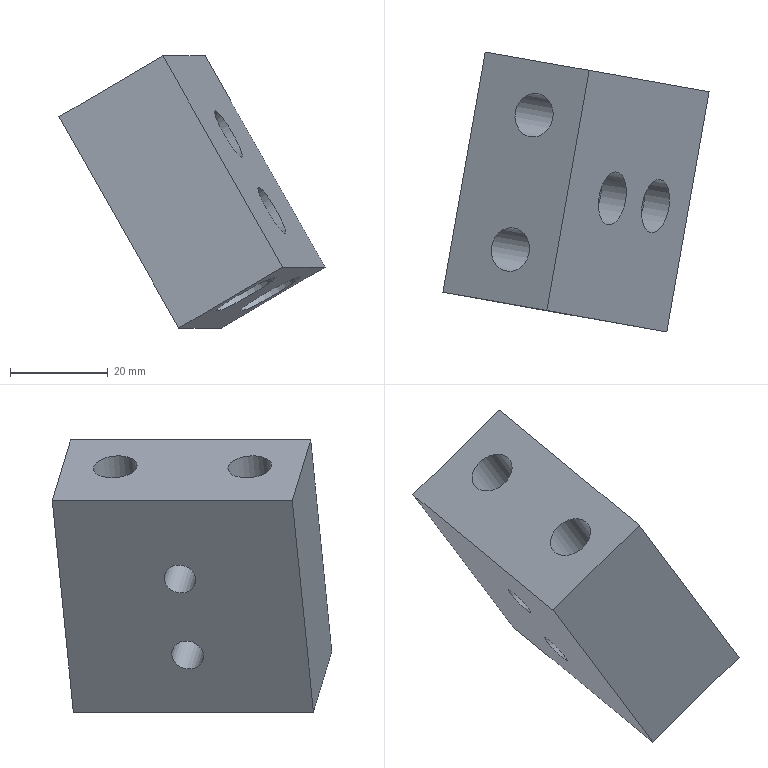Part | NX | features solid 2 | 1 solid | 18 faces | box 54.624 x 57.341 x 55.801 mm | volume 52253 mm3 | plane 10 | cylinder 8 | commonest cylinder face diameters 6.6 x2 9 x2 11 x2 14 x2
STEP:
#1=CARTESIAN_POINT('',(-861.482,388.099,62.179));
#2=VERTEX_POINT('',#1);
#3=CARTESIAN_POINT('',(-852.8,437.34,62.179));
#4=VERTEX_POINT('',#3);
#5=CARTESIAN_POINT('',(-851.845,442.756,62.179));
#6=DIRECTION('',(0.1736,0.9848,0.));
#7=VECTOR('',#6,1000.);
#8=LINE('',#5,#7);
#9=EDGE_CURVE('',#2,#4,#8,.T.);
#10=ORIENTED_EDGE('',*,*,#9,.F.);
#11=CARTESIAN_POINT('',(-836.862,383.758,18.877));
#12=VERTEX_POINT('',#11);
#13=CARTESIAN_POINT('',(-823.567,381.414,-4.505));
#14=DIRECTION('',(-0.4924,0.08682,0.866));
#15=VECTOR('',#14,1000.);
#16=LINE('',#13,#15);
#17=EDGE_CURVE('',#12,#2,#16,.T.);
#18=ORIENTED_EDGE('',*,*,#17,.F.);
#19=CARTESIAN_POINT('',(-828.18,432.998,18.877));
#20=VERTEX_POINT('',#19);
#21=CARTESIAN_POINT('',(-836.862,383.758,18.877));
#22=DIRECTION('',(0.1736,0.9848,0.));
#23=VECTOR('',#22,1000.);
#24=LINE('',#21,#23);
#25=EDGE_CURVE('',#12,#20,#24,.T.);
#26=ORIENTED_EDGE('',*,*,#25,.T.);
#27=CARTESIAN_POINT('',(-814.885,430.654,-4.505));
#28=DIRECTION('',(-0.4924,0.08682,0.866));
#29=VECTOR('',#28,1000.);
#30=LINE('',#27,#29);
#31=EDGE_CURVE('',#20,#4,#30,.T.);
#32=ORIENTED_EDGE('',*,*,#31,.T.);
#33=EDGE_LOOP('',(#10,#18,#26,#32));
#34=FACE_BOUND('',#33,.T.);
#35=CARTESIAN_POINT('',(-838.213,414.967,30.569));
#36=VERTEX_POINT('',#35);
#37=CARTESIAN_POINT('',(-839.168,409.55,30.569));
#38=DIRECTION('',(-0.8529,0.1504,-0.5));
#39=DIRECTION('',(0.1736,0.9848,0.));
#40=AXIS2_PLACEMENT_3D('',#37,#38,#39);
#41=CIRCLE('',#40,5.5);
#42=EDGE_CURVE('',#36,#36,#41,.T.);
#43=ORIENTED_EDGE('',*,*,#42,.T.);
#44=EDGE_LOOP('',(#43));
#45=FACE_BOUND('',#44,.T.);
#46=CARTESIAN_POINT('',(-845.324,410.636,41.394));
#47=VERTEX_POINT('',#46);
#48=CARTESIAN_POINT('',(-848.032,411.113,46.157));
#49=DIRECTION('',(0.8529,-0.1504,0.5));
#50=DIRECTION('',(0.4924,-0.08682,-0.866));
#51=AXIS2_PLACEMENT_3D('',#48,#49,#50);
#52=CIRCLE('',#51,5.5);
#53=EDGE_CURVE('',#47,#47,#52,.F.);
#54=ORIENTED_EDGE('',*,*,#53,.T.);
#55=EDGE_LOOP('',(#54));
#56=FACE_BOUND('',#55,.T.);
#57=CARTESIAN_POINT('',(-823.567,381.414,-4.505));
#58=DIRECTION('',(0.8529,-0.1504,0.5));
#59=DIRECTION('',(-0.1736,-0.9848,0.));
#60=AXIS2_PLACEMENT_3D('',#57,#58,#59);
#61=PLANE('',#60);
#62=ADVANCED_FACE('',(#34,#45,#56),#61,.T.);
#63=CARTESIAN_POINT('',(-849.502,436.758,6.377));
#64=VERTEX_POINT('',#63);
#65=CARTESIAN_POINT('',(-828.18,432.998,18.877));
#66=DIRECTION('',(-0.8529,0.1504,-0.5));
#67=VECTOR('',#66,1000.);
#68=LINE('',#65,#67);
#69=EDGE_CURVE('',#20,#64,#68,.T.);
#70=ORIENTED_EDGE('',*,*,#69,.F.);
#71=ORIENTED_EDGE('',*,*,#25,.F.);
#72=CARTESIAN_POINT('',(-858.184,387.518,6.377));
#73=VERTEX_POINT('',#72);
#74=CARTESIAN_POINT('',(-836.862,383.758,18.877));
#75=DIRECTION('',(0.8529,-0.1504,0.5));
#76=VECTOR('',#75,1000.);
#77=LINE('',#74,#76);
#78=EDGE_CURVE('',#73,#12,#77,.T.);
#79=ORIENTED_EDGE('',*,*,#78,.F.);
#80=CARTESIAN_POINT('',(-858.184,387.518,6.377));
#81=DIRECTION('',(-0.1736,-0.9848,0.));
#82=VECTOR('',#81,1000.);
#83=LINE('',#80,#82);
#84=EDGE_CURVE('',#64,#73,#83,.T.);
#85=ORIENTED_EDGE('',*,*,#84,.F.);
#86=EDGE_LOOP('',(#70,#71,#79,#85));
#87=FACE_BOUND('',#86,.T.);
#88=CARTESIAN_POINT('',(-833.501,422.767,16.877));
#89=VERTEX_POINT('',#88);
#90=CARTESIAN_POINT('',(-839.471,423.82,13.377));
#91=DIRECTION('',(-0.4924,0.08682,0.866));
#92=DIRECTION('',(0.8529,-0.1504,0.5));
#93=AXIS2_PLACEMENT_3D('',#90,#91,#92);
#94=CIRCLE('',#93,7.);
#95=EDGE_CURVE('',#89,#89,#94,.T.);
#96=ORIENTED_EDGE('',*,*,#95,.T.);
#97=EDGE_LOOP('',(#96));
#98=FACE_BOUND('',#97,.T.);
#99=CARTESIAN_POINT('',(-838.364,395.192,16.877));
#100=VERTEX_POINT('',#99);
#101=CARTESIAN_POINT('',(-844.334,396.245,13.377));
#102=DIRECTION('',(-0.4924,0.08682,0.866));
#103=DIRECTION('',(0.8529,-0.1504,0.5));
#104=AXIS2_PLACEMENT_3D('',#101,#102,#103);
#105=CIRCLE('',#104,7.);
#106=EDGE_CURVE('',#100,#100,#105,.T.);
#107=ORIENTED_EDGE('',*,*,#106,.T.);
#108=EDGE_LOOP('',(#107));
#109=FACE_BOUND('',#108,.T.);
#110=CARTESIAN_POINT('',(-836.862,383.758,18.877));
#111=DIRECTION('',(-0.4924,0.08682,0.866));
#112=DIRECTION('',(0.1736,0.9848,0.));
#113=AXIS2_PLACEMENT_3D('',#110,#111,#112);
#114=PLANE('',#113);
#115=ADVANCED_FACE('',(#87,#98,#109),#114,.F.);
#116=CARTESIAN_POINT('',(-882.804,391.859,49.679));
#117=VERTEX_POINT('',#116);
#118=CARTESIAN_POINT('',(-992.909,411.273,-14.871));
#119=DIRECTION('',(0.8529,-0.1504,0.5));
#120=VECTOR('',#119,1000.);
#121=LINE('',#118,#120);
#122=EDGE_CURVE('',#117,#2,#121,.T.);
#123=ORIENTED_EDGE('',*,*,#122,.F.);
#124=CARTESIAN_POINT('',(-844.889,385.173,-17.005));
#125=DIRECTION('',(-0.4924,0.08682,0.866));
#126=VECTOR('',#125,1000.);
#127=LINE('',#124,#126);
#128=EDGE_CURVE('',#73,#117,#127,.T.);
#129=ORIENTED_EDGE('',*,*,#128,.F.);
#130=ORIENTED_EDGE('',*,*,#78,.T.);
#131=ORIENTED_EDGE('',*,*,#17,.T.);
#132=EDGE_LOOP('',(#123,#129,#130,#131));
#133=FACE_BOUND('',#132,.T.);
#134=CARTESIAN_POINT('',(-844.889,385.173,-17.005));
#135=DIRECTION('',(-0.1736,-0.9848,0.));
#136=DIRECTION('',(-0.8529,0.1504,-0.5));
#137=AXIS2_PLACEMENT_3D('',#134,#135,#136);
#138=PLANE('',#137);
#139=ADVANCED_FACE('',(#133),#138,.T.);
#140=CARTESIAN_POINT('',(-874.122,441.099,49.679));
#141=VERTEX_POINT('',#140);
#142=CARTESIAN_POINT('',(-984.227,460.514,-14.871));
#143=DIRECTION('',(-0.8529,0.1504,-0.5));
#144=VECTOR('',#143,1000.);
#145=LINE('',#142,#144);
#146=EDGE_CURVE('',#4,#141,#145,.T.);
#147=ORIENTED_EDGE('',*,*,#146,.F.);
#148=ORIENTED_EDGE('',*,*,#31,.F.);
#149=ORIENTED_EDGE('',*,*,#69,.T.);
#150=CARTESIAN_POINT('',(-836.207,434.414,-17.005));
#151=DIRECTION('',(-0.4924,0.08682,0.866));
#152=VECTOR('',#151,1000.);
#153=LINE('',#150,#152);
#154=EDGE_CURVE('',#64,#141,#153,.T.);
#155=ORIENTED_EDGE('',*,*,#154,.T.);
#156=EDGE_LOOP('',(#147,#148,#149,#155));
#157=FACE_BOUND('',#156,.T.);
#158=CARTESIAN_POINT('',(-814.885,430.654,-4.505));
#159=DIRECTION('',(0.1736,0.9848,0.));
#160=DIRECTION('',(0.8529,-0.1504,0.5));
#161=AXIS2_PLACEMENT_3D('',#158,#159,#160);
#162=PLANE('',#161);
#163=ADVANCED_FACE('',(#157),#162,.T.);
#164=CARTESIAN_POINT('',(-870.978,415.159,36.515));
#165=VERTEX_POINT('',#164);
#166=CARTESIAN_POINT('',(-869.353,414.873,33.657));
#167=DIRECTION('',(-0.8529,0.1504,-0.5));
#168=DIRECTION('',(-0.4924,0.08682,0.866));
#169=AXIS2_PLACEMENT_3D('',#166,#167,#168);
#170=CIRCLE('',#169,3.3);
#171=EDGE_CURVE('',#165,#165,#170,.T.);
#172=ORIENTED_EDGE('',*,*,#171,.F.);
#173=EDGE_LOOP('',(#172));
#174=FACE_BOUND('',#173,.T.);
#175=CARTESIAN_POINT('',(-859.917,416.56,18.069));
#176=VERTEX_POINT('',#175);
#177=CARTESIAN_POINT('',(-860.49,413.31,18.069));
#178=DIRECTION('',(-0.8529,0.1504,-0.5));
#179=DIRECTION('',(0.1736,0.9848,0.));
#180=AXIS2_PLACEMENT_3D('',#177,#178,#179);
#181=CIRCLE('',#180,3.3);
#182=EDGE_CURVE('',#176,#176,#181,.T.);
#183=ORIENTED_EDGE('',*,*,#182,.F.);
#184=EDGE_LOOP('',(#183));
#185=FACE_BOUND('',#184,.T.);
#186=CARTESIAN_POINT('',(-873.167,446.516,49.679));
#187=DIRECTION('',(-0.1736,-0.9848,0.));
#188=VECTOR('',#187,1000.);
#189=LINE('',#186,#188);
#190=EDGE_CURVE('',#141,#117,#189,.T.);
#191=ORIENTED_EDGE('',*,*,#190,.F.);
#192=ORIENTED_EDGE('',*,*,#154,.F.);
#193=ORIENTED_EDGE('',*,*,#84,.T.);
#194=ORIENTED_EDGE('',*,*,#128,.T.);
#195=EDGE_LOOP('',(#191,#192,#193,#194));
#196=FACE_BOUND('',#195,.T.);
#197=CARTESIAN_POINT('',(-836.207,434.414,-17.005));
#198=DIRECTION('',(-0.8529,0.1504,-0.5));
#199=DIRECTION('',(0.1736,0.9848,0.));
#200=AXIS2_PLACEMENT_3D('',#197,#198,#199);
#201=PLANE('',#200);
#202=ADVANCED_FACE('',(#174,#185,#196),#201,.T.);
#203=CARTESIAN_POINT('',(-860.254,427.484,58.929));
#204=VERTEX_POINT('',#203);
#205=CARTESIAN_POINT('',(-864.092,428.161,56.679));
#206=DIRECTION('',(-0.4924,0.08682,0.866));
#207=DIRECTION('',(0.8529,-0.1504,0.5));
#208=AXIS2_PLACEMENT_3D('',#205,#206,#207);
#209=CIRCLE('',#208,4.5);
#210=EDGE_CURVE('',#204,#204,#209,.T.);
#211=ORIENTED_EDGE('',*,*,#210,.F.);
#212=EDGE_LOOP('',(#211));
#213=FACE_BOUND('',#212,.T.);
#214=CARTESIAN_POINT('',(-865.116,399.91,58.929));
#215=VERTEX_POINT('',#214);
#216=CARTESIAN_POINT('',(-868.954,400.586,56.679));
#217=DIRECTION('',(-0.4924,0.08682,0.866));
#218=DIRECTION('',(0.8529,-0.1504,0.5));
#219=AXIS2_PLACEMENT_3D('',#216,#217,#218);
#220=CIRCLE('',#219,4.5);
#221=EDGE_CURVE('',#215,#215,#220,.T.);
#222=ORIENTED_EDGE('',*,*,#221,.F.);
#223=EDGE_LOOP('',(#222));
#224=FACE_BOUND('',#223,.T.);
#225=ORIENTED_EDGE('',*,*,#122,.T.);
#226=ORIENTED_EDGE('',*,*,#9,.T.);
#227=ORIENTED_EDGE('',*,*,#146,.T.);
#228=ORIENTED_EDGE('',*,*,#190,.T.);
#229=EDGE_LOOP('',(#225,#226,#227,#228));
#230=FACE_BOUND('',#229,.T.);
#231=CARTESIAN_POINT('',(-983.272,465.93,-14.871));
#232=DIRECTION('',(-0.4924,0.08682,0.866));
#233=DIRECTION('',(0.1736,0.9848,0.));
#234=AXIS2_PLACEMENT_3D('',#231,#232,#233);
#235=PLANE('',#234);
#236=ADVANCED_FACE('',(#213,#224,#230),#235,.T.);
#237=ORIENTED_EDGE('',*,*,#182,.T.);
#238=EDGE_LOOP('',(#237));
#239=FACE_BOUND('',#238,.T.);
#240=CARTESIAN_POINT('',(-843.713,413.702,27.569));
#241=VERTEX_POINT('',#240);
#242=CARTESIAN_POINT('',(-844.286,410.453,27.569));
#243=DIRECTION('',(-0.8529,0.1504,-0.5));
#244=DIRECTION('',(0.1736,0.9848,0.));
#245=AXIS2_PLACEMENT_3D('',#242,#243,#244);
#246=CIRCLE('',#245,3.3);
#247=EDGE_CURVE('',#241,#241,#246,.T.);
#248=ORIENTED_EDGE('',*,*,#247,.F.);
#249=EDGE_LOOP('',(#248));
#250=FACE_BOUND('',#249,.T.);
#251=CARTESIAN_POINT('',(-881.812,417.07,5.569));
#252=DIRECTION('',(-0.8529,0.1504,-0.5));
#253=DIRECTION('',(0.1736,0.9848,0.));
#254=AXIS2_PLACEMENT_3D('',#251,#252,#253);
#255=CYLINDRICAL_SURFACE('',#254,3.3);
#256=ADVANCED_FACE('',(#239,#250),#255,.F.);
#257=ORIENTED_EDGE('',*,*,#247,.T.);
#258=EDGE_LOOP('',(#257));
#259=FACE_BOUND('',#258,.T.);
#260=CARTESIAN_POINT('',(-843.331,415.869,27.569));
#261=VERTEX_POINT('',#260);
#262=CARTESIAN_POINT('',(-844.286,410.453,27.569));
#263=DIRECTION('',(-0.8529,0.1504,-0.5));
#264=DIRECTION('',(0.1736,0.9848,0.));
#265=AXIS2_PLACEMENT_3D('',#262,#263,#264);
#266=CIRCLE('',#265,5.5);
#267=EDGE_CURVE('',#261,#261,#266,.T.);
#268=ORIENTED_EDGE('',*,*,#267,.F.);
#269=EDGE_LOOP('',(#268));
#270=FACE_BOUND('',#269,.T.);
#271=CARTESIAN_POINT('',(-844.039,410.409,27.136));
#272=DIRECTION('',(-0.8529,0.1504,-0.5));
#273=DIRECTION('',(0.1736,0.9848,0.));
#274=AXIS2_PLACEMENT_3D('',#271,#272,#273);
#275=PLANE('',#274);
#276=ADVANCED_FACE('',(#259,#270),#275,.F.);
#277=ORIENTED_EDGE('',*,*,#267,.T.);
#278=EDGE_LOOP('',(#277));
#279=FACE_BOUND('',#278,.T.);
#280=ORIENTED_EDGE('',*,*,#42,.F.);
#281=EDGE_LOOP('',(#280));
#282=FACE_BOUND('',#281,.T.);
#283=CARTESIAN_POINT('',(-839.168,409.55,30.569));
#284=DIRECTION('',(-0.8529,0.1504,-0.5));
#285=DIRECTION('',(0.1736,0.9848,0.));
#286=AXIS2_PLACEMENT_3D('',#283,#284,#285);
#287=CYLINDRICAL_SURFACE('',#286,5.5);
#288=ADVANCED_FACE('',(#279,#282),#287,.F.);
#289=ORIENTED_EDGE('',*,*,#221,.T.);
#290=EDGE_LOOP('',(#289));
#291=FACE_BOUND('',#290,.T.);
#292=CARTESIAN_POINT('',(-844.435,396.263,22.556));
#293=VERTEX_POINT('',#292);
#294=CARTESIAN_POINT('',(-848.273,396.94,20.306));
#295=DIRECTION('',(-0.4924,0.08682,0.866));
#296=DIRECTION('',(0.8529,-0.1504,0.5));
#297=AXIS2_PLACEMENT_3D('',#294,#295,#296);
#298=CIRCLE('',#297,4.5);
#299=EDGE_CURVE('',#293,#293,#298,.T.);
#300=ORIENTED_EDGE('',*,*,#299,.F.);
#301=EDGE_LOOP('',(#300));
#302=FACE_BOUND('',#301,.T.);
#303=CARTESIAN_POINT('',(-880.279,402.583,76.597));
#304=DIRECTION('',(-0.4924,0.08682,0.866));
#305=DIRECTION('',(0.1736,0.9848,0.));
#306=AXIS2_PLACEMENT_3D('',#303,#304,#305);
#307=CYLINDRICAL_SURFACE('',#306,4.5);
#308=ADVANCED_FACE('',(#291,#302),#307,.F.);
#309=ORIENTED_EDGE('',*,*,#299,.T.);
#310=EDGE_LOOP('',(#309));
#311=FACE_BOUND('',#310,.T.);
#312=CARTESIAN_POINT('',(-842.303,395.887,23.806));
#313=VERTEX_POINT('',#312);
#314=CARTESIAN_POINT('',(-848.273,396.94,20.306));
#315=DIRECTION('',(-0.4924,0.08682,0.866));
#316=DIRECTION('',(0.8529,-0.1504,0.5));
#317=AXIS2_PLACEMENT_3D('',#314,#315,#316);
#318=CIRCLE('',#317,7.);
#319=EDGE_CURVE('',#313,#313,#318,.T.);
#320=ORIENTED_EDGE('',*,*,#319,.F.);
#321=EDGE_LOOP('',(#320));
#322=FACE_BOUND('',#321,.T.);
#323=CARTESIAN_POINT('',(-848.273,396.94,20.306));
#324=DIRECTION('',(-0.4924,0.08682,0.866));
#325=DIRECTION('',(0.1736,0.9848,0.));
#326=AXIS2_PLACEMENT_3D('',#323,#324,#325);
#327=PLANE('',#326);
#328=ADVANCED_FACE('',(#311,#322),#327,.F.);
#329=ORIENTED_EDGE('',*,*,#319,.T.);
#330=EDGE_LOOP('',(#329));
#331=FACE_BOUND('',#330,.T.);
#332=ORIENTED_EDGE('',*,*,#106,.F.);
#333=EDGE_LOOP('',(#332));
#334=FACE_BOUND('',#333,.T.);
#335=CARTESIAN_POINT('',(-831.039,393.901,-10.005));
#336=DIRECTION('',(-0.4924,0.08682,0.866));
#337=DIRECTION('',(0.1736,0.9848,0.));
#338=AXIS2_PLACEMENT_3D('',#335,#336,#337);
#339=CYLINDRICAL_SURFACE('',#338,7.);
#340=ADVANCED_FACE('',(#331,#334),#339,.F.);
#341=ORIENTED_EDGE('',*,*,#210,.T.);
#342=EDGE_LOOP('',(#341));
#343=FACE_BOUND('',#342,.T.);
#344=CARTESIAN_POINT('',(-839.573,423.838,22.556));
#345=VERTEX_POINT('',#344);
#346=CARTESIAN_POINT('',(-843.411,424.514,20.306));
#347=DIRECTION('',(-0.4924,0.08682,0.866));
#348=DIRECTION('',(0.8529,-0.1504,0.5));
#349=AXIS2_PLACEMENT_3D('',#346,#347,#348);
#350=CIRCLE('',#349,4.5);
#351=EDGE_CURVE('',#345,#345,#350,.T.);
#352=ORIENTED_EDGE('',*,*,#351,.F.);
#353=EDGE_LOOP('',(#352));
#354=FACE_BOUND('',#353,.T.);
#355=CARTESIAN_POINT('',(-875.417,430.158,76.597));
#356=DIRECTION('',(-0.4924,0.08682,0.866));
#357=DIRECTION('',(0.1736,0.9848,0.));
#358=AXIS2_PLACEMENT_3D('',#355,#356,#357);
#359=CYLINDRICAL_SURFACE('',#358,4.5);
#360=ADVANCED_FACE('',(#343,#354),#359,.F.);
#361=ORIENTED_EDGE('',*,*,#351,.T.);
#362=EDGE_LOOP('',(#361));
#363=FACE_BOUND('',#362,.T.);
#364=CARTESIAN_POINT('',(-837.441,423.462,23.806));
#365=VERTEX_POINT('',#364);
#366=CARTESIAN_POINT('',(-843.411,424.514,20.306));
#367=DIRECTION('',(-0.4924,0.08682,0.866));
#368=DIRECTION('',(0.8529,-0.1504,0.5));
#369=AXIS2_PLACEMENT_3D('',#366,#367,#368);
#370=CIRCLE('',#369,7.);
#371=EDGE_CURVE('',#365,#365,#370,.T.);
#372=ORIENTED_EDGE('',*,*,#371,.F.);
#373=EDGE_LOOP('',(#372));
#374=FACE_BOUND('',#373,.T.);
#375=CARTESIAN_POINT('',(-843.411,424.514,20.306));
#376=DIRECTION('',(-0.4924,0.08682,0.866));
#377=DIRECTION('',(0.1736,0.9848,0.));
#378=AXIS2_PLACEMENT_3D('',#375,#376,#377);
#379=PLANE('',#378);
#380=ADVANCED_FACE('',(#363,#374),#379,.F.);
#381=ORIENTED_EDGE('',*,*,#371,.T.);
#382=EDGE_LOOP('',(#381));
#383=FACE_BOUND('',#382,.T.);
#384=ORIENTED_EDGE('',*,*,#95,.F.);
#385=EDGE_LOOP('',(#384));
#386=FACE_BOUND('',#385,.T.);
#387=CARTESIAN_POINT('',(-826.177,421.475,-10.005));
#388=DIRECTION('',(-0.4924,0.08682,0.866));
#389=DIRECTION('',(0.1736,0.9848,0.));
#390=AXIS2_PLACEMENT_3D('',#387,#388,#389);
#391=CYLINDRICAL_SURFACE('',#390,7.);
#392=ADVANCED_FACE('',(#383,#386),#391,.F.);
#393=ORIENTED_EDGE('',*,*,#171,.T.);
#394=EDGE_LOOP('',(#393));
#395=FACE_BOUND('',#394,.T.);
#396=CARTESIAN_POINT('',(-854.774,412.302,46.015));
#397=VERTEX_POINT('',#396);
#398=CARTESIAN_POINT('',(-853.149,412.015,43.157));
#399=DIRECTION('',(-0.8529,0.1504,-0.5));
#400=DIRECTION('',(-0.4924,0.08682,0.866));
#401=AXIS2_PLACEMENT_3D('',#398,#399,#400);
#402=CIRCLE('',#401,3.3);
#403=EDGE_CURVE('',#397,#397,#402,.F.);
#404=ORIENTED_EDGE('',*,*,#403,.T.);
#405=EDGE_LOOP('',(#404));
#406=FACE_BOUND('',#405,.T.);
#407=CARTESIAN_POINT('',(-853.149,412.015,43.157));
#408=DIRECTION('',(-0.8529,0.1504,-0.5));
#409=DIRECTION('',(-0.4924,0.08682,0.866));
#410=AXIS2_PLACEMENT_3D('',#407,#408,#409);
#411=CYLINDRICAL_SURFACE('',#410,3.3);
#412=ADVANCED_FACE('',(#395,#406),#411,.F.);
#413=ORIENTED_EDGE('',*,*,#53,.F.);
#414=EDGE_LOOP('',(#413));
#415=FACE_BOUND('',#414,.T.);
#416=CARTESIAN_POINT('',(-852.194,417.432,43.157));
#417=VERTEX_POINT('',#416);
#418=CARTESIAN_POINT('',(-853.149,412.015,43.157));
#419=DIRECTION('',(-0.8529,0.1504,-0.5));
#420=DIRECTION('',(0.1736,0.9848,0.));
#421=AXIS2_PLACEMENT_3D('',#418,#419,#420);
#422=CIRCLE('',#421,5.5);
#423=EDGE_CURVE('',#417,#417,#422,.T.);
#424=ORIENTED_EDGE('',*,*,#423,.T.);
#425=EDGE_LOOP('',(#424));
#426=FACE_BOUND('',#425,.T.);
#427=CARTESIAN_POINT('',(-853.149,412.015,43.157));
#428=DIRECTION('',(0.8529,-0.1504,0.5));
#429=DIRECTION('',(0.4924,-0.08682,-0.866));
#430=AXIS2_PLACEMENT_3D('',#427,#428,#429);
#431=CYLINDRICAL_SURFACE('',#430,5.5);
#432=ADVANCED_FACE('',(#415,#426),#431,.F.);
#433=ORIENTED_EDGE('',*,*,#403,.F.);
#434=EDGE_LOOP('',(#433));
#435=FACE_BOUND('',#434,.T.);
#436=ORIENTED_EDGE('',*,*,#423,.F.);
#437=EDGE_LOOP('',(#436));
#438=FACE_BOUND('',#437,.T.);
#439=CARTESIAN_POINT('',(-853.149,412.015,43.157));
#440=DIRECTION('',(-0.8529,0.1504,-0.5));
#441=DIRECTION('',(-0.4924,0.08682,0.866));
#442=AXIS2_PLACEMENT_3D('',#439,#440,#441);
#443=PLANE('',#442);
#444=ADVANCED_FACE('',(#435,#438),#443,.F.);
#445=CLOSED_SHELL('',(#62,#115,#139,#163,#202,#236,#256,#276,#288,#308,#328,#340,#360,#380,#392,#412,#432,#444));
#446=MANIFOLD_SOLID_BREP('',#445);
#447=(LENGTH_UNIT()NAMED_UNIT(*)SI_UNIT(.MILLI.,.METRE.));
#448=UNCERTAINTY_MEASURE_WITH_UNIT(LENGTH_MEASURE(0.00001),#447,'','');
#449=(NAMED_UNIT(*)PLANE_ANGLE_UNIT()SI_UNIT($,.RADIAN.));
#450=(NAMED_UNIT(*)SI_UNIT($,.STERADIAN.)SOLID_ANGLE_UNIT());
#451=(GEOMETRIC_REPRESENTATION_CONTEXT(3)GLOBAL_UNCERTAINTY_ASSIGNED_CONTEXT((#448))GLOBAL_UNIT_ASSIGNED_CONTEXT((#447,#449,#450))REPRESENTATION_CONTEXT('',''));
#452=ADVANCED_BREP_SHAPE_REPRESENTATION('',(#446),#451);